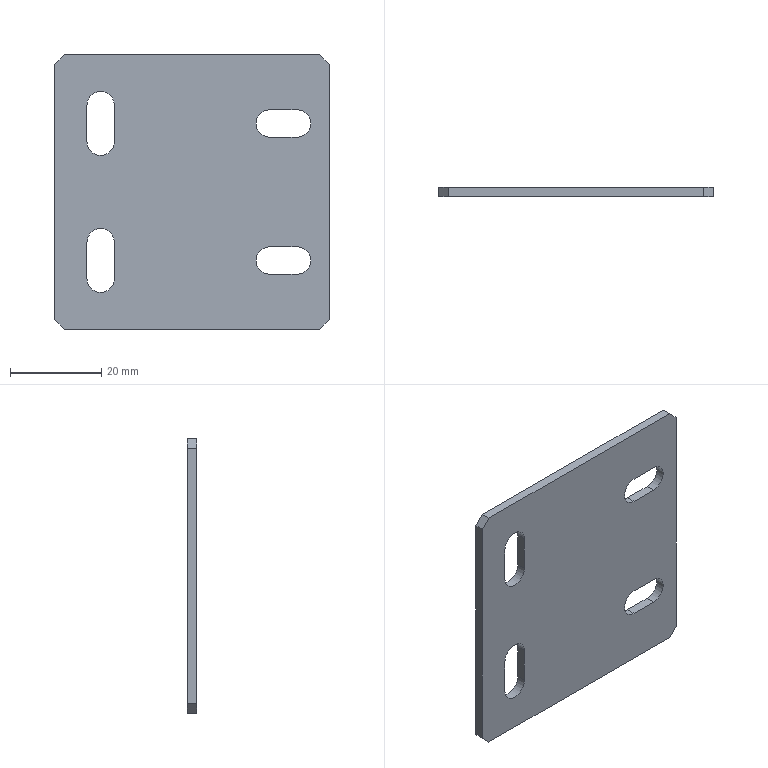Part | NX | features BREP 1 | 1 solid | 28 faces | box 60 x 2 x 60 mm | volume 6622 mm3 | plane 18 | cylinder 10 | commonest cylinder face diameters 6 x10
STEP:
#1=CARTESIAN_POINT('',(30.,-2.,28.));
#2=VERTEX_POINT('',#1);
#3=CARTESIAN_POINT('',(28.,-2.,30.));
#4=VERTEX_POINT('',#3);
#5=CARTESIAN_POINT('',(28.,-2.,30.));
#6=DIRECTION('',(-0.7071,0.,0.7071));
#7=VECTOR('',#6,1000.);
#8=LINE('',#5,#7);
#9=EDGE_CURVE('',#2,#4,#8,.T.);
#10=ORIENTED_EDGE('',*,*,#9,.F.);
#11=CARTESIAN_POINT('',(30.,0.,28.));
#12=VERTEX_POINT('',#11);
#13=CARTESIAN_POINT('',(30.,-2.,28.));
#14=DIRECTION('',(0.,-1.,0.));
#15=VECTOR('',#14,1000.);
#16=LINE('',#13,#15);
#17=EDGE_CURVE('',#12,#2,#16,.T.);
#18=ORIENTED_EDGE('',*,*,#17,.F.);
#19=CARTESIAN_POINT('',(28.,0.,30.));
#20=VERTEX_POINT('',#19);
#21=CARTESIAN_POINT('',(29.,0.,29.));
#22=DIRECTION('',(0.7071,0.,-0.7071));
#23=VECTOR('',#22,1000.);
#24=LINE('',#21,#23);
#25=EDGE_CURVE('',#20,#12,#24,.T.);
#26=ORIENTED_EDGE('',*,*,#25,.F.);
#27=CARTESIAN_POINT('',(28.,-2.,30.));
#28=DIRECTION('',(0.,1.,0.));
#29=VECTOR('',#28,1000.);
#30=LINE('',#27,#29);
#31=EDGE_CURVE('',#4,#20,#30,.T.);
#32=ORIENTED_EDGE('',*,*,#31,.F.);
#33=EDGE_LOOP('',(#10,#18,#26,#32));
#34=FACE_BOUND('',#33,.T.);
#35=CARTESIAN_POINT('',(28.,-2.,30.));
#36=DIRECTION('',(-0.7071,0.,-0.7071));
#37=DIRECTION('',(0.,1.,0.));
#38=AXIS2_PLACEMENT_3D('',#35,#36,#37);
#39=PLANE('',#38);
#40=ADVANCED_FACE('',(#34),#39,.F.);
#41=CARTESIAN_POINT('',(28.,-2.,-30.));
#42=VERTEX_POINT('',#41);
#43=CARTESIAN_POINT('',(30.,-2.,-28.));
#44=VERTEX_POINT('',#43);
#45=CARTESIAN_POINT('',(30.,-2.,-28.));
#46=DIRECTION('',(0.7071,0.,0.7071));
#47=VECTOR('',#46,1000.);
#48=LINE('',#45,#47);
#49=EDGE_CURVE('',#42,#44,#48,.T.);
#50=ORIENTED_EDGE('',*,*,#49,.F.);
#51=CARTESIAN_POINT('',(28.,0.,-30.));
#52=VERTEX_POINT('',#51);
#53=CARTESIAN_POINT('',(28.,-2.,-30.));
#54=DIRECTION('',(0.,-1.,0.));
#55=VECTOR('',#54,1000.);
#56=LINE('',#53,#55);
#57=EDGE_CURVE('',#52,#42,#56,.T.);
#58=ORIENTED_EDGE('',*,*,#57,.F.);
#59=CARTESIAN_POINT('',(30.,0.,-28.));
#60=VERTEX_POINT('',#59);
#61=CARTESIAN_POINT('',(29.,0.,-29.));
#62=DIRECTION('',(-0.7071,0.,-0.7071));
#63=VECTOR('',#62,1000.);
#64=LINE('',#61,#63);
#65=EDGE_CURVE('',#60,#52,#64,.T.);
#66=ORIENTED_EDGE('',*,*,#65,.F.);
#67=CARTESIAN_POINT('',(30.,-2.,-28.));
#68=DIRECTION('',(0.,1.,0.));
#69=VECTOR('',#68,1000.);
#70=LINE('',#67,#69);
#71=EDGE_CURVE('',#44,#60,#70,.T.);
#72=ORIENTED_EDGE('',*,*,#71,.F.);
#73=EDGE_LOOP('',(#50,#58,#66,#72));
#74=FACE_BOUND('',#73,.T.);
#75=CARTESIAN_POINT('',(30.,-2.,-28.));
#76=DIRECTION('',(-0.7071,0.,0.7071));
#77=DIRECTION('',(0.,1.,0.));
#78=AXIS2_PLACEMENT_3D('',#75,#76,#77);
#79=PLANE('',#78);
#80=ADVANCED_FACE('',(#74),#79,.F.);
#81=CARTESIAN_POINT('',(-30.,-2.,-28.));
#82=VERTEX_POINT('',#81);
#83=CARTESIAN_POINT('',(-28.,-2.,-30.));
#84=VERTEX_POINT('',#83);
#85=CARTESIAN_POINT('',(-28.,-2.,-30.));
#86=DIRECTION('',(0.7071,0.,-0.7071));
#87=VECTOR('',#86,1000.);
#88=LINE('',#85,#87);
#89=EDGE_CURVE('',#82,#84,#88,.T.);
#90=ORIENTED_EDGE('',*,*,#89,.F.);
#91=CARTESIAN_POINT('',(-30.,0.,-28.));
#92=VERTEX_POINT('',#91);
#93=CARTESIAN_POINT('',(-30.,-2.,-28.));
#94=DIRECTION('',(0.,-1.,0.));
#95=VECTOR('',#94,1000.);
#96=LINE('',#93,#95);
#97=EDGE_CURVE('',#92,#82,#96,.T.);
#98=ORIENTED_EDGE('',*,*,#97,.F.);
#99=CARTESIAN_POINT('',(-28.,0.,-30.));
#100=VERTEX_POINT('',#99);
#101=CARTESIAN_POINT('',(-29.,0.,-29.));
#102=DIRECTION('',(-0.7071,0.,0.7071));
#103=VECTOR('',#102,1000.);
#104=LINE('',#101,#103);
#105=EDGE_CURVE('',#100,#92,#104,.T.);
#106=ORIENTED_EDGE('',*,*,#105,.F.);
#107=CARTESIAN_POINT('',(-28.,-2.,-30.));
#108=DIRECTION('',(0.,1.,0.));
#109=VECTOR('',#108,1000.);
#110=LINE('',#107,#109);
#111=EDGE_CURVE('',#84,#100,#110,.T.);
#112=ORIENTED_EDGE('',*,*,#111,.F.);
#113=EDGE_LOOP('',(#90,#98,#106,#112));
#114=FACE_BOUND('',#113,.T.);
#115=CARTESIAN_POINT('',(-28.,-2.,-30.));
#116=DIRECTION('',(0.7071,0.,0.7071));
#117=DIRECTION('',(0.,1.,0.));
#118=AXIS2_PLACEMENT_3D('',#115,#116,#117);
#119=PLANE('',#118);
#120=ADVANCED_FACE('',(#114),#119,.F.);
#121=CARTESIAN_POINT('',(-28.,-2.,30.));
#122=VERTEX_POINT('',#121);
#123=CARTESIAN_POINT('',(-30.,-2.,28.));
#124=VERTEX_POINT('',#123);
#125=CARTESIAN_POINT('',(-30.,-2.,28.));
#126=DIRECTION('',(-0.7071,0.,-0.7071));
#127=VECTOR('',#126,1000.);
#128=LINE('',#125,#127);
#129=EDGE_CURVE('',#122,#124,#128,.T.);
#130=ORIENTED_EDGE('',*,*,#129,.F.);
#131=CARTESIAN_POINT('',(-28.,0.,30.));
#132=VERTEX_POINT('',#131);
#133=CARTESIAN_POINT('',(-28.,-2.,30.));
#134=DIRECTION('',(0.,-1.,0.));
#135=VECTOR('',#134,1000.);
#136=LINE('',#133,#135);
#137=EDGE_CURVE('',#132,#122,#136,.T.);
#138=ORIENTED_EDGE('',*,*,#137,.F.);
#139=CARTESIAN_POINT('',(-30.,0.,28.));
#140=VERTEX_POINT('',#139);
#141=CARTESIAN_POINT('',(-29.,0.,29.));
#142=DIRECTION('',(0.7071,0.,0.7071));
#143=VECTOR('',#142,1000.);
#144=LINE('',#141,#143);
#145=EDGE_CURVE('',#140,#132,#144,.T.);
#146=ORIENTED_EDGE('',*,*,#145,.F.);
#147=CARTESIAN_POINT('',(-30.,-2.,28.));
#148=DIRECTION('',(0.,1.,0.));
#149=VECTOR('',#148,1000.);
#150=LINE('',#147,#149);
#151=EDGE_CURVE('',#124,#140,#150,.T.);
#152=ORIENTED_EDGE('',*,*,#151,.F.);
#153=EDGE_LOOP('',(#130,#138,#146,#152));
#154=FACE_BOUND('',#153,.T.);
#155=CARTESIAN_POINT('',(-30.,-2.,28.));
#156=DIRECTION('',(0.7071,0.,-0.7071));
#157=DIRECTION('',(0.,1.,0.));
#158=AXIS2_PLACEMENT_3D('',#155,#156,#157);
#159=PLANE('',#158);
#160=ADVANCED_FACE('',(#154),#159,.F.);
#161=CARTESIAN_POINT('',(-17.,0.,-19.));
#162=VERTEX_POINT('',#161);
#163=CARTESIAN_POINT('',(-17.,-2.,-19.));
#164=VERTEX_POINT('',#163);
#165=CARTESIAN_POINT('',(-17.,-2.,-19.));
#166=DIRECTION('',(0.,-1.,0.));
#167=VECTOR('',#166,1000.);
#168=LINE('',#165,#167);
#169=EDGE_CURVE('',#162,#164,#168,.T.);
#170=ORIENTED_EDGE('',*,*,#169,.T.);
#171=CARTESIAN_POINT('',(-17.,-2.,-11.));
#172=VERTEX_POINT('',#171);
#173=CARTESIAN_POINT('',(-17.,-2.,-11.));
#174=DIRECTION('',(0.,0.,-1.));
#175=VECTOR('',#174,1000.);
#176=LINE('',#173,#175);
#177=EDGE_CURVE('',#172,#164,#176,.T.);
#178=ORIENTED_EDGE('',*,*,#177,.F.);
#179=CARTESIAN_POINT('',(-17.,0.,-11.));
#180=VERTEX_POINT('',#179);
#181=CARTESIAN_POINT('',(-17.,-2.,-11.));
#182=DIRECTION('',(0.,-1.,0.));
#183=VECTOR('',#182,1000.);
#184=LINE('',#181,#183);
#185=EDGE_CURVE('',#180,#172,#184,.T.);
#186=ORIENTED_EDGE('',*,*,#185,.F.);
#187=CARTESIAN_POINT('',(-17.,0.,-11.));
#188=DIRECTION('',(0.,0.,-1.));
#189=VECTOR('',#188,1000.);
#190=LINE('',#187,#189);
#191=EDGE_CURVE('',#180,#162,#190,.T.);
#192=ORIENTED_EDGE('',*,*,#191,.T.);
#193=EDGE_LOOP('',(#170,#178,#186,#192));
#194=FACE_BOUND('',#193,.T.);
#195=CARTESIAN_POINT('',(-17.,-2.,-11.));
#196=DIRECTION('',(1.,0.,0.));
#197=DIRECTION('',(0.,1.,0.));
#198=AXIS2_PLACEMENT_3D('',#195,#196,#197);
#199=PLANE('',#198);
#200=ADVANCED_FACE('',(#194),#199,.F.);
#201=CARTESIAN_POINT('',(-23.,-2.,-19.));
#202=VERTEX_POINT('',#201);
#203=CARTESIAN_POINT('',(-23.,0.,-19.));
#204=VERTEX_POINT('',#203);
#205=CARTESIAN_POINT('',(-23.,0.,-19.));
#206=DIRECTION('',(0.,1.,0.));
#207=VECTOR('',#206,1000.);
#208=LINE('',#205,#207);
#209=EDGE_CURVE('',#202,#204,#208,.T.);
#210=ORIENTED_EDGE('',*,*,#209,.T.);
#211=CARTESIAN_POINT('',(-23.,0.,-11.));
#212=VERTEX_POINT('',#211);
#213=CARTESIAN_POINT('',(-23.,0.,-11.));
#214=DIRECTION('',(0.,0.,-1.));
#215=VECTOR('',#214,1000.);
#216=LINE('',#213,#215);
#217=EDGE_CURVE('',#212,#204,#216,.T.);
#218=ORIENTED_EDGE('',*,*,#217,.F.);
#219=CARTESIAN_POINT('',(-23.,-2.,-11.));
#220=VERTEX_POINT('',#219);
#221=CARTESIAN_POINT('',(-23.,0.,-11.));
#222=DIRECTION('',(0.,-1.,0.));
#223=VECTOR('',#222,1000.);
#224=LINE('',#221,#223);
#225=EDGE_CURVE('',#212,#220,#224,.T.);
#226=ORIENTED_EDGE('',*,*,#225,.T.);
#227=CARTESIAN_POINT('',(-23.,-2.,-11.));
#228=DIRECTION('',(0.,0.,-1.));
#229=VECTOR('',#228,1000.);
#230=LINE('',#227,#229);
#231=EDGE_CURVE('',#220,#202,#230,.T.);
#232=ORIENTED_EDGE('',*,*,#231,.T.);
#233=EDGE_LOOP('',(#210,#218,#226,#232));
#234=FACE_BOUND('',#233,.T.);
#235=CARTESIAN_POINT('',(-23.,0.,-11.));
#236=DIRECTION('',(-1.,0.,0.));
#237=DIRECTION('',(0.,0.,1.));
#238=AXIS2_PLACEMENT_3D('',#235,#236,#237);
#239=PLANE('',#238);
#240=ADVANCED_FACE('',(#234),#239,.F.);
#241=CARTESIAN_POINT('',(-20.,-2.,-8.));
#242=VERTEX_POINT('',#241);
#243=CARTESIAN_POINT('',(-20.,0.,-8.));
#244=VERTEX_POINT('',#243);
#245=CARTESIAN_POINT('',(-20.,0.,-8.));
#246=DIRECTION('',(0.,1.,0.));
#247=VECTOR('',#246,1000.);
#248=LINE('',#245,#247);
#249=EDGE_CURVE('',#242,#244,#248,.T.);
#250=ORIENTED_EDGE('',*,*,#249,.F.);
#251=CARTESIAN_POINT('',(-20.,-2.,-11.));
#252=DIRECTION('',(0.,1.,0.));
#253=DIRECTION('',(0.,0.,1.));
#254=AXIS2_PLACEMENT_3D('',#251,#252,#253);
#255=CIRCLE('',#254,3.);
#256=EDGE_CURVE('',#220,#242,#255,.T.);
#257=ORIENTED_EDGE('',*,*,#256,.F.);
#258=ORIENTED_EDGE('',*,*,#225,.F.);
#259=CARTESIAN_POINT('',(-20.,0.,-11.));
#260=DIRECTION('',(0.,1.,0.));
#261=DIRECTION('',(0.,0.,1.));
#262=AXIS2_PLACEMENT_3D('',#259,#260,#261);
#263=CIRCLE('',#262,3.);
#264=EDGE_CURVE('',#212,#244,#263,.T.);
#265=ORIENTED_EDGE('',*,*,#264,.T.);
#266=EDGE_LOOP('',(#250,#257,#258,#265));
#267=FACE_BOUND('',#266,.T.);
#268=CARTESIAN_POINT('',(-20.,0.,-11.));
#269=DIRECTION('',(0.,1.,0.));
#270=DIRECTION('',(0.,0.,1.));
#271=AXIS2_PLACEMENT_3D('',#268,#269,#270);
#272=CYLINDRICAL_SURFACE('',#271,3.);
#273=ADVANCED_FACE('',(#267),#272,.F.);
#274=CARTESIAN_POINT('',(-20.,-2.,-19.));
#275=DIRECTION('',(0.,1.,0.));
#276=DIRECTION('',(0.,0.,1.));
#277=AXIS2_PLACEMENT_3D('',#274,#275,#276);
#278=CIRCLE('',#277,3.);
#279=EDGE_CURVE('',#164,#202,#278,.T.);
#280=ORIENTED_EDGE('',*,*,#279,.F.);
#281=ORIENTED_EDGE('',*,*,#169,.F.);
#282=CARTESIAN_POINT('',(-20.,0.,-19.));
#283=DIRECTION('',(0.,1.,0.));
#284=DIRECTION('',(0.,0.,1.));
#285=AXIS2_PLACEMENT_3D('',#282,#283,#284);
#286=CIRCLE('',#285,3.);
#287=EDGE_CURVE('',#162,#204,#286,.T.);
#288=ORIENTED_EDGE('',*,*,#287,.T.);
#289=ORIENTED_EDGE('',*,*,#209,.F.);
#290=EDGE_LOOP('',(#280,#281,#288,#289));
#291=FACE_BOUND('',#290,.T.);
#292=CARTESIAN_POINT('',(-20.,0.,-19.));
#293=DIRECTION('',(0.,1.,0.));
#294=DIRECTION('',(0.,0.,1.));
#295=AXIS2_PLACEMENT_3D('',#292,#293,#294);
#296=CYLINDRICAL_SURFACE('',#295,3.);
#297=ADVANCED_FACE('',(#291),#296,.F.);
#298=CARTESIAN_POINT('',(-17.,0.,11.));
#299=VERTEX_POINT('',#298);
#300=CARTESIAN_POINT('',(-17.,-2.,11.));
#301=VERTEX_POINT('',#300);
#302=CARTESIAN_POINT('',(-17.,-2.,11.));
#303=DIRECTION('',(0.,-1.,0.));
#304=VECTOR('',#303,1000.);
#305=LINE('',#302,#304);
#306=EDGE_CURVE('',#299,#301,#305,.T.);
#307=ORIENTED_EDGE('',*,*,#306,.T.);
#308=CARTESIAN_POINT('',(-17.,-2.,19.));
#309=VERTEX_POINT('',#308);
#310=CARTESIAN_POINT('',(-17.,-2.,19.));
#311=DIRECTION('',(0.,0.,-1.));
#312=VECTOR('',#311,1000.);
#313=LINE('',#310,#312);
#314=EDGE_CURVE('',#309,#301,#313,.T.);
#315=ORIENTED_EDGE('',*,*,#314,.F.);
#316=CARTESIAN_POINT('',(-17.,0.,19.));
#317=VERTEX_POINT('',#316);
#318=CARTESIAN_POINT('',(-17.,-2.,19.));
#319=DIRECTION('',(0.,-1.,0.));
#320=VECTOR('',#319,1000.);
#321=LINE('',#318,#320);
#322=EDGE_CURVE('',#317,#309,#321,.T.);
#323=ORIENTED_EDGE('',*,*,#322,.F.);
#324=CARTESIAN_POINT('',(-17.,0.,19.));
#325=DIRECTION('',(0.,0.,-1.));
#326=VECTOR('',#325,1000.);
#327=LINE('',#324,#326);
#328=EDGE_CURVE('',#317,#299,#327,.T.);
#329=ORIENTED_EDGE('',*,*,#328,.T.);
#330=EDGE_LOOP('',(#307,#315,#323,#329));
#331=FACE_BOUND('',#330,.T.);
#332=CARTESIAN_POINT('',(-17.,-2.,19.));
#333=DIRECTION('',(1.,0.,0.));
#334=DIRECTION('',(0.,1.,0.));
#335=AXIS2_PLACEMENT_3D('',#332,#333,#334);
#336=PLANE('',#335);
#337=ADVANCED_FACE('',(#331),#336,.F.);
#338=CARTESIAN_POINT('',(-23.,-2.,11.));
#339=VERTEX_POINT('',#338);
#340=CARTESIAN_POINT('',(-23.,0.,11.));
#341=VERTEX_POINT('',#340);
#342=CARTESIAN_POINT('',(-23.,0.,11.));
#343=DIRECTION('',(0.,1.,0.));
#344=VECTOR('',#343,1000.);
#345=LINE('',#342,#344);
#346=EDGE_CURVE('',#339,#341,#345,.T.);
#347=ORIENTED_EDGE('',*,*,#346,.T.);
#348=CARTESIAN_POINT('',(-23.,0.,19.));
#349=VERTEX_POINT('',#348);
#350=CARTESIAN_POINT('',(-23.,0.,19.));
#351=DIRECTION('',(0.,0.,-1.));
#352=VECTOR('',#351,1000.);
#353=LINE('',#350,#352);
#354=EDGE_CURVE('',#349,#341,#353,.T.);
#355=ORIENTED_EDGE('',*,*,#354,.F.);
#356=CARTESIAN_POINT('',(-23.,-2.,19.));
#357=VERTEX_POINT('',#356);
#358=CARTESIAN_POINT('',(-23.,0.,19.));
#359=DIRECTION('',(0.,-1.,0.));
#360=VECTOR('',#359,1000.);
#361=LINE('',#358,#360);
#362=EDGE_CURVE('',#349,#357,#361,.T.);
#363=ORIENTED_EDGE('',*,*,#362,.T.);
#364=CARTESIAN_POINT('',(-23.,-2.,19.));
#365=DIRECTION('',(0.,0.,-1.));
#366=VECTOR('',#365,1000.);
#367=LINE('',#364,#366);
#368=EDGE_CURVE('',#357,#339,#367,.T.);
#369=ORIENTED_EDGE('',*,*,#368,.T.);
#370=EDGE_LOOP('',(#347,#355,#363,#369));
#371=FACE_BOUND('',#370,.T.);
#372=CARTESIAN_POINT('',(-23.,0.,19.));
#373=DIRECTION('',(-1.,0.,0.));
#374=DIRECTION('',(0.,0.,1.));
#375=AXIS2_PLACEMENT_3D('',#372,#373,#374);
#376=PLANE('',#375);
#377=ADVANCED_FACE('',(#371),#376,.F.);
#378=CARTESIAN_POINT('',(-20.,-2.,22.));
#379=VERTEX_POINT('',#378);
#380=CARTESIAN_POINT('',(-20.,0.,22.));
#381=VERTEX_POINT('',#380);
#382=CARTESIAN_POINT('',(-20.,0.,22.));
#383=DIRECTION('',(0.,1.,0.));
#384=VECTOR('',#383,1000.);
#385=LINE('',#382,#384);
#386=EDGE_CURVE('',#379,#381,#385,.T.);
#387=ORIENTED_EDGE('',*,*,#386,.F.);
#388=CARTESIAN_POINT('',(-20.,-2.,19.));
#389=DIRECTION('',(0.,1.,0.));
#390=DIRECTION('',(0.,0.,1.));
#391=AXIS2_PLACEMENT_3D('',#388,#389,#390);
#392=CIRCLE('',#391,3.);
#393=EDGE_CURVE('',#357,#379,#392,.T.);
#394=ORIENTED_EDGE('',*,*,#393,.F.);
#395=ORIENTED_EDGE('',*,*,#362,.F.);
#396=CARTESIAN_POINT('',(-20.,0.,19.));
#397=DIRECTION('',(0.,1.,0.));
#398=DIRECTION('',(0.,0.,1.));
#399=AXIS2_PLACEMENT_3D('',#396,#397,#398);
#400=CIRCLE('',#399,3.);
#401=EDGE_CURVE('',#349,#381,#400,.T.);
#402=ORIENTED_EDGE('',*,*,#401,.T.);
#403=EDGE_LOOP('',(#387,#394,#395,#402));
#404=FACE_BOUND('',#403,.T.);
#405=CARTESIAN_POINT('',(-20.,0.,19.));
#406=DIRECTION('',(0.,1.,0.));
#407=DIRECTION('',(0.,0.,1.));
#408=AXIS2_PLACEMENT_3D('',#405,#406,#407);
#409=CYLINDRICAL_SURFACE('',#408,3.);
#410=ADVANCED_FACE('',(#404),#409,.F.);
#411=CARTESIAN_POINT('',(-20.,-2.,11.));
#412=DIRECTION('',(0.,1.,0.));
#413=DIRECTION('',(0.,0.,1.));
#414=AXIS2_PLACEMENT_3D('',#411,#412,#413);
#415=CIRCLE('',#414,3.);
#416=EDGE_CURVE('',#301,#339,#415,.T.);
#417=ORIENTED_EDGE('',*,*,#416,.F.);
#418=ORIENTED_EDGE('',*,*,#306,.F.);
#419=CARTESIAN_POINT('',(-20.,0.,11.));
#420=DIRECTION('',(0.,1.,0.));
#421=DIRECTION('',(0.,0.,1.));
#422=AXIS2_PLACEMENT_3D('',#419,#420,#421);
#423=CIRCLE('',#422,3.);
#424=EDGE_CURVE('',#299,#341,#423,.T.);
#425=ORIENTED_EDGE('',*,*,#424,.T.);
#426=ORIENTED_EDGE('',*,*,#346,.F.);
#427=EDGE_LOOP('',(#417,#418,#425,#426));
#428=FACE_BOUND('',#427,.T.);
#429=CARTESIAN_POINT('',(-20.,0.,11.));
#430=DIRECTION('',(0.,1.,0.));
#431=DIRECTION('',(0.,0.,1.));
#432=AXIS2_PLACEMENT_3D('',#429,#430,#431);
#433=CYLINDRICAL_SURFACE('',#432,3.);
#434=ADVANCED_FACE('',(#428),#433,.F.);
#435=CARTESIAN_POINT('',(23.,0.,-12.));
#436=VERTEX_POINT('',#435);
#437=CARTESIAN_POINT('',(23.,-2.,-12.));
#438=VERTEX_POINT('',#437);
#439=CARTESIAN_POINT('',(23.,0.,-12.));
#440=DIRECTION('',(0.,-1.,0.));
#441=VECTOR('',#440,1000.);
#442=LINE('',#439,#441);
#443=EDGE_CURVE('',#436,#438,#442,.T.);
#444=ORIENTED_EDGE('',*,*,#443,.T.);
#445=CARTESIAN_POINT('',(17.,-2.,-12.));
#446=VERTEX_POINT('',#445);
#447=CARTESIAN_POINT('',(17.,-2.,-12.));
#448=DIRECTION('',(1.,0.,0.));
#449=VECTOR('',#448,1000.);
#450=LINE('',#447,#449);
#451=EDGE_CURVE('',#446,#438,#450,.T.);
#452=ORIENTED_EDGE('',*,*,#451,.F.);
#453=CARTESIAN_POINT('',(17.,0.,-12.));
#454=VERTEX_POINT('',#453);
#455=CARTESIAN_POINT('',(17.,0.,-12.));
#456=DIRECTION('',(0.,1.,0.));
#457=VECTOR('',#456,1000.);
#458=LINE('',#455,#457);
#459=EDGE_CURVE('',#446,#454,#458,.T.);
#460=ORIENTED_EDGE('',*,*,#459,.T.);
#461=CARTESIAN_POINT('',(17.,0.,-12.));
#462=DIRECTION('',(1.,0.,0.));
#463=VECTOR('',#462,1000.);
#464=LINE('',#461,#463);
#465=EDGE_CURVE('',#454,#436,#464,.T.);
#466=ORIENTED_EDGE('',*,*,#465,.T.);
#467=EDGE_LOOP('',(#444,#452,#460,#466));
#468=FACE_BOUND('',#467,.T.);
#469=CARTESIAN_POINT('',(17.,0.,-12.));
#470=DIRECTION('',(0.,0.,1.));
#471=DIRECTION('',(1.,0.,0.));
#472=AXIS2_PLACEMENT_3D('',#469,#470,#471);
#473=PLANE('',#472);
#474=ADVANCED_FACE('',(#468),#473,.F.);
#475=CARTESIAN_POINT('',(23.,-2.,-18.));
#476=VERTEX_POINT('',#475);
#477=CARTESIAN_POINT('',(23.,0.,-18.));
#478=VERTEX_POINT('',#477);
#479=CARTESIAN_POINT('',(23.,0.,-18.));
#480=DIRECTION('',(0.,1.,0.));
#481=VECTOR('',#480,1000.);
#482=LINE('',#479,#481);
#483=EDGE_CURVE('',#476,#478,#482,.T.);
#484=ORIENTED_EDGE('',*,*,#483,.T.);
#485=CARTESIAN_POINT('',(17.,0.,-18.));
#486=VERTEX_POINT('',#485);
#487=CARTESIAN_POINT('',(17.,0.,-18.));
#488=DIRECTION('',(1.,0.,0.));
#489=VECTOR('',#488,1000.);
#490=LINE('',#487,#489);
#491=EDGE_CURVE('',#486,#478,#490,.T.);
#492=ORIENTED_EDGE('',*,*,#491,.F.);
#493=CARTESIAN_POINT('',(17.,-2.,-18.));
#494=VERTEX_POINT('',#493);
#495=CARTESIAN_POINT('',(17.,0.,-18.));
#496=DIRECTION('',(0.,-1.,0.));
#497=VECTOR('',#496,1000.);
#498=LINE('',#495,#497);
#499=EDGE_CURVE('',#486,#494,#498,.T.);
#500=ORIENTED_EDGE('',*,*,#499,.T.);
#501=CARTESIAN_POINT('',(17.,-2.,-18.));
#502=DIRECTION('',(1.,0.,0.));
#503=VECTOR('',#502,1000.);
#504=LINE('',#501,#503);
#505=EDGE_CURVE('',#494,#476,#504,.T.);
#506=ORIENTED_EDGE('',*,*,#505,.T.);
#507=EDGE_LOOP('',(#484,#492,#500,#506));
#508=FACE_BOUND('',#507,.T.);
#509=CARTESIAN_POINT('',(17.,0.,-18.));
#510=DIRECTION('',(0.,0.,-1.));
#511=DIRECTION('',(-1.,0.,0.));
#512=AXIS2_PLACEMENT_3D('',#509,#510,#511);
#513=PLANE('',#512);
#514=ADVANCED_FACE('',(#508),#513,.F.);
#515=CARTESIAN_POINT('',(17.,0.,-15.));
#516=DIRECTION('',(0.,1.,0.));
#517=DIRECTION('',(0.,0.,1.));
#518=AXIS2_PLACEMENT_3D('',#515,#516,#517);
#519=CIRCLE('',#518,3.);
#520=EDGE_CURVE('',#486,#454,#519,.T.);
#521=ORIENTED_EDGE('',*,*,#520,.T.);
#522=ORIENTED_EDGE('',*,*,#459,.F.);
#523=CARTESIAN_POINT('',(17.,-2.,-15.));
#524=DIRECTION('',(0.,1.,0.));
#525=DIRECTION('',(0.,0.,1.));
#526=AXIS2_PLACEMENT_3D('',#523,#524,#525);
#527=CIRCLE('',#526,3.);
#528=EDGE_CURVE('',#494,#446,#527,.T.);
#529=ORIENTED_EDGE('',*,*,#528,.F.);
#530=ORIENTED_EDGE('',*,*,#499,.F.);
#531=EDGE_LOOP('',(#521,#522,#529,#530));
#532=FACE_BOUND('',#531,.T.);
#533=CARTESIAN_POINT('',(17.,0.,-15.));
#534=DIRECTION('',(0.,1.,0.));
#535=DIRECTION('',(0.,0.,1.));
#536=AXIS2_PLACEMENT_3D('',#533,#534,#535);
#537=CYLINDRICAL_SURFACE('',#536,3.);
#538=ADVANCED_FACE('',(#532),#537,.F.);
#539=CARTESIAN_POINT('',(23.,-2.,-15.));
#540=DIRECTION('',(0.,1.,0.));
#541=DIRECTION('',(0.,0.,1.));
#542=AXIS2_PLACEMENT_3D('',#539,#540,#541);
#543=CIRCLE('',#542,3.);
#544=EDGE_CURVE('',#438,#476,#543,.T.);
#545=ORIENTED_EDGE('',*,*,#544,.F.);
#546=ORIENTED_EDGE('',*,*,#443,.F.);
#547=CARTESIAN_POINT('',(23.,0.,-15.));
#548=DIRECTION('',(0.,1.,0.));
#549=DIRECTION('',(0.,0.,1.));
#550=AXIS2_PLACEMENT_3D('',#547,#548,#549);
#551=CIRCLE('',#550,3.);
#552=EDGE_CURVE('',#436,#478,#551,.T.);
#553=ORIENTED_EDGE('',*,*,#552,.T.);
#554=ORIENTED_EDGE('',*,*,#483,.F.);
#555=EDGE_LOOP('',(#545,#546,#553,#554));
#556=FACE_BOUND('',#555,.T.);
#557=CARTESIAN_POINT('',(23.,0.,-15.));
#558=DIRECTION('',(0.,1.,0.));
#559=DIRECTION('',(0.,0.,1.));
#560=AXIS2_PLACEMENT_3D('',#557,#558,#559);
#561=CYLINDRICAL_SURFACE('',#560,3.);
#562=ADVANCED_FACE('',(#556),#561,.F.);
#563=CARTESIAN_POINT('',(23.,0.,18.));
#564=VERTEX_POINT('',#563);
#565=CARTESIAN_POINT('',(23.,-2.,18.));
#566=VERTEX_POINT('',#565);
#567=CARTESIAN_POINT('',(23.,0.,18.));
#568=DIRECTION('',(0.,-1.,0.));
#569=VECTOR('',#568,1000.);
#570=LINE('',#567,#569);
#571=EDGE_CURVE('',#564,#566,#570,.T.);
#572=ORIENTED_EDGE('',*,*,#571,.T.);
#573=CARTESIAN_POINT('',(17.,-2.,18.));
#574=VERTEX_POINT('',#573);
#575=CARTESIAN_POINT('',(17.,-2.,18.));
#576=DIRECTION('',(1.,0.,0.));
#577=VECTOR('',#576,1000.);
#578=LINE('',#575,#577);
#579=EDGE_CURVE('',#574,#566,#578,.T.);
#580=ORIENTED_EDGE('',*,*,#579,.F.);
#581=CARTESIAN_POINT('',(17.,0.,18.));
#582=VERTEX_POINT('',#581);
#583=CARTESIAN_POINT('',(17.,0.,18.));
#584=DIRECTION('',(0.,1.,0.));
#585=VECTOR('',#584,1000.);
#586=LINE('',#583,#585);
#587=EDGE_CURVE('',#574,#582,#586,.T.);
#588=ORIENTED_EDGE('',*,*,#587,.T.);
#589=CARTESIAN_POINT('',(17.,0.,18.));
#590=DIRECTION('',(1.,0.,0.));
#591=VECTOR('',#590,1000.);
#592=LINE('',#589,#591);
#593=EDGE_CURVE('',#582,#564,#592,.T.);
#594=ORIENTED_EDGE('',*,*,#593,.T.);
#595=EDGE_LOOP('',(#572,#580,#588,#594));
#596=FACE_BOUND('',#595,.T.);
#597=CARTESIAN_POINT('',(17.,0.,18.));
#598=DIRECTION('',(0.,0.,1.));
#599=DIRECTION('',(1.,0.,0.));
#600=AXIS2_PLACEMENT_3D('',#597,#598,#599);
#601=PLANE('',#600);
#602=ADVANCED_FACE('',(#596),#601,.F.);
#603=CARTESIAN_POINT('',(23.,-2.,12.));
#604=VERTEX_POINT('',#603);
#605=CARTESIAN_POINT('',(23.,0.,12.));
#606=VERTEX_POINT('',#605);
#607=CARTESIAN_POINT('',(23.,0.,12.));
#608=DIRECTION('',(0.,1.,0.));
#609=VECTOR('',#608,1000.);
#610=LINE('',#607,#609);
#611=EDGE_CURVE('',#604,#606,#610,.T.);
#612=ORIENTED_EDGE('',*,*,#611,.T.);
#613=CARTESIAN_POINT('',(17.,0.,12.));
#614=VERTEX_POINT('',#613);
#615=CARTESIAN_POINT('',(17.,0.,12.));
#616=DIRECTION('',(1.,0.,0.));
#617=VECTOR('',#616,1000.);
#618=LINE('',#615,#617);
#619=EDGE_CURVE('',#614,#606,#618,.T.);
#620=ORIENTED_EDGE('',*,*,#619,.F.);
#621=CARTESIAN_POINT('',(17.,-2.,12.));
#622=VERTEX_POINT('',#621);
#623=CARTESIAN_POINT('',(17.,0.,12.));
#624=DIRECTION('',(0.,-1.,0.));
#625=VECTOR('',#624,1000.);
#626=LINE('',#623,#625);
#627=EDGE_CURVE('',#614,#622,#626,.T.);
#628=ORIENTED_EDGE('',*,*,#627,.T.);
#629=CARTESIAN_POINT('',(17.,-2.,12.));
#630=DIRECTION('',(1.,0.,0.));
#631=VECTOR('',#630,1000.);
#632=LINE('',#629,#631);
#633=EDGE_CURVE('',#622,#604,#632,.T.);
#634=ORIENTED_EDGE('',*,*,#633,.T.);
#635=EDGE_LOOP('',(#612,#620,#628,#634));
#636=FACE_BOUND('',#635,.T.);
#637=CARTESIAN_POINT('',(17.,0.,12.));
#638=DIRECTION('',(0.,0.,-1.));
#639=DIRECTION('',(-1.,0.,0.));
#640=AXIS2_PLACEMENT_3D('',#637,#638,#639);
#641=PLANE('',#640);
#642=ADVANCED_FACE('',(#636),#641,.F.);
#643=CARTESIAN_POINT('',(17.,0.,15.));
#644=DIRECTION('',(0.,1.,0.));
#645=DIRECTION('',(0.,0.,1.));
#646=AXIS2_PLACEMENT_3D('',#643,#644,#645);
#647=CIRCLE('',#646,3.);
#648=EDGE_CURVE('',#614,#582,#647,.T.);
#649=ORIENTED_EDGE('',*,*,#648,.T.);
#650=ORIENTED_EDGE('',*,*,#587,.F.);
#651=CARTESIAN_POINT('',(17.,-2.,15.));
#652=DIRECTION('',(0.,1.,0.));
#653=DIRECTION('',(0.,0.,1.));
#654=AXIS2_PLACEMENT_3D('',#651,#652,#653);
#655=CIRCLE('',#654,3.);
#656=EDGE_CURVE('',#622,#574,#655,.T.);
#657=ORIENTED_EDGE('',*,*,#656,.F.);
#658=ORIENTED_EDGE('',*,*,#627,.F.);
#659=EDGE_LOOP('',(#649,#650,#657,#658));
#660=FACE_BOUND('',#659,.T.);
#661=CARTESIAN_POINT('',(17.,0.,15.));
#662=DIRECTION('',(0.,1.,0.));
#663=DIRECTION('',(0.,0.,1.));
#664=AXIS2_PLACEMENT_3D('',#661,#662,#663);
#665=CYLINDRICAL_SURFACE('',#664,3.);
#666=ADVANCED_FACE('',(#660),#665,.F.);
#667=CARTESIAN_POINT('',(23.,-2.,15.));
#668=DIRECTION('',(0.,1.,0.));
#669=DIRECTION('',(0.,0.,1.));
#670=AXIS2_PLACEMENT_3D('',#667,#668,#669);
#671=CIRCLE('',#670,3.);
#672=EDGE_CURVE('',#566,#604,#671,.T.);
#673=ORIENTED_EDGE('',*,*,#672,.F.);
#674=ORIENTED_EDGE('',*,*,#571,.F.);
#675=CARTESIAN_POINT('',(23.,0.,15.));
#676=DIRECTION('',(0.,1.,0.));
#677=DIRECTION('',(0.,0.,1.));
#678=AXIS2_PLACEMENT_3D('',#675,#676,#677);
#679=CIRCLE('',#678,3.);
#680=EDGE_CURVE('',#564,#606,#679,.T.);
#681=ORIENTED_EDGE('',*,*,#680,.T.);
#682=ORIENTED_EDGE('',*,*,#611,.F.);
#683=EDGE_LOOP('',(#673,#674,#681,#682));
#684=FACE_BOUND('',#683,.T.);
#685=CARTESIAN_POINT('',(23.,0.,15.));
#686=DIRECTION('',(0.,1.,0.));
#687=DIRECTION('',(0.,0.,1.));
#688=AXIS2_PLACEMENT_3D('',#685,#686,#687);
#689=CYLINDRICAL_SURFACE('',#688,3.);
#690=ADVANCED_FACE('',(#684),#689,.F.);
#691=CARTESIAN_POINT('',(30.,0.,30.));
#692=DIRECTION('',(1.,0.,0.));
#693=VECTOR('',#692,1000.);
#694=LINE('',#691,#693);
#695=EDGE_CURVE('',#132,#20,#694,.T.);
#696=ORIENTED_EDGE('',*,*,#695,.F.);
#697=ORIENTED_EDGE('',*,*,#137,.T.);
#698=CARTESIAN_POINT('',(30.,-2.,30.));
#699=DIRECTION('',(1.,0.,0.));
#700=VECTOR('',#699,1000.);
#701=LINE('',#698,#700);
#702=EDGE_CURVE('',#122,#4,#701,.T.);
#703=ORIENTED_EDGE('',*,*,#702,.T.);
#704=ORIENTED_EDGE('',*,*,#31,.T.);
#705=EDGE_LOOP('',(#696,#697,#703,#704));
#706=FACE_BOUND('',#705,.T.);
#707=CARTESIAN_POINT('',(30.,-2.,30.));
#708=DIRECTION('',(0.,0.,1.));
#709=DIRECTION('',(1.,0.,0.));
#710=AXIS2_PLACEMENT_3D('',#707,#708,#709);
#711=PLANE('',#710);
#712=ADVANCED_FACE('',(#706),#711,.T.);
#713=CARTESIAN_POINT('',(30.,-2.,30.));
#714=DIRECTION('',(0.,0.,-1.));
#715=VECTOR('',#714,1000.);
#716=LINE('',#713,#715);
#717=EDGE_CURVE('',#2,#44,#716,.T.);
#718=ORIENTED_EDGE('',*,*,#717,.T.);
#719=ORIENTED_EDGE('',*,*,#71,.T.);
#720=CARTESIAN_POINT('',(30.,0.,30.));
#721=DIRECTION('',(0.,0.,-1.));
#722=VECTOR('',#721,1000.);
#723=LINE('',#720,#722);
#724=EDGE_CURVE('',#12,#60,#723,.T.);
#725=ORIENTED_EDGE('',*,*,#724,.F.);
#726=ORIENTED_EDGE('',*,*,#17,.T.);
#727=EDGE_LOOP('',(#718,#719,#725,#726));
#728=FACE_BOUND('',#727,.T.);
#729=CARTESIAN_POINT('',(30.,-2.,30.));
#730=DIRECTION('',(1.,0.,0.));
#731=DIRECTION('',(0.,0.,-1.));
#732=AXIS2_PLACEMENT_3D('',#729,#730,#731);
#733=PLANE('',#732);
#734=ADVANCED_FACE('',(#728),#733,.T.);
#735=CARTESIAN_POINT('',(30.,-2.,-30.));
#736=DIRECTION('',(-1.,0.,0.));
#737=VECTOR('',#736,1000.);
#738=LINE('',#735,#737);
#739=EDGE_CURVE('',#42,#84,#738,.T.);
#740=ORIENTED_EDGE('',*,*,#739,.T.);
#741=ORIENTED_EDGE('',*,*,#111,.T.);
#742=CARTESIAN_POINT('',(30.,0.,-30.));
#743=DIRECTION('',(-1.,0.,0.));
#744=VECTOR('',#743,1000.);
#745=LINE('',#742,#744);
#746=EDGE_CURVE('',#52,#100,#745,.T.);
#747=ORIENTED_EDGE('',*,*,#746,.F.);
#748=ORIENTED_EDGE('',*,*,#57,.T.);
#749=EDGE_LOOP('',(#740,#741,#747,#748));
#750=FACE_BOUND('',#749,.T.);
#751=CARTESIAN_POINT('',(30.,-2.,-30.));
#752=DIRECTION('',(0.,0.,-1.));
#753=DIRECTION('',(-1.,0.,0.));
#754=AXIS2_PLACEMENT_3D('',#751,#752,#753);
#755=PLANE('',#754);
#756=ADVANCED_FACE('',(#750),#755,.T.);
#757=CARTESIAN_POINT('',(-30.,-2.,30.));
#758=DIRECTION('',(0.,0.,1.));
#759=VECTOR('',#758,1000.);
#760=LINE('',#757,#759);
#761=EDGE_CURVE('',#82,#124,#760,.T.);
#762=ORIENTED_EDGE('',*,*,#761,.T.);
#763=ORIENTED_EDGE('',*,*,#151,.T.);
#764=CARTESIAN_POINT('',(-30.,0.,30.));
#765=DIRECTION('',(0.,0.,1.));
#766=VECTOR('',#765,1000.);
#767=LINE('',#764,#766);
#768=EDGE_CURVE('',#92,#140,#767,.T.);
#769=ORIENTED_EDGE('',*,*,#768,.F.);
#770=ORIENTED_EDGE('',*,*,#97,.T.);
#771=EDGE_LOOP('',(#762,#763,#769,#770));
#772=FACE_BOUND('',#771,.T.);
#773=CARTESIAN_POINT('',(-30.,-2.,30.));
#774=DIRECTION('',(-1.,0.,0.));
#775=DIRECTION('',(0.,0.,1.));
#776=AXIS2_PLACEMENT_3D('',#773,#774,#775);
#777=PLANE('',#776);
#778=ADVANCED_FACE('',(#772),#777,.T.);
#779=ORIENTED_EDGE('',*,*,#505,.F.);
#780=ORIENTED_EDGE('',*,*,#528,.T.);
#781=ORIENTED_EDGE('',*,*,#451,.T.);
#782=ORIENTED_EDGE('',*,*,#544,.T.);
#783=EDGE_LOOP('',(#779,#780,#781,#782));
#784=FACE_BOUND('',#783,.T.);
#785=ORIENTED_EDGE('',*,*,#702,.F.);
#786=ORIENTED_EDGE('',*,*,#129,.T.);
#787=ORIENTED_EDGE('',*,*,#761,.F.);
#788=ORIENTED_EDGE('',*,*,#89,.T.);
#789=ORIENTED_EDGE('',*,*,#739,.F.);
#790=ORIENTED_EDGE('',*,*,#49,.T.);
#791=ORIENTED_EDGE('',*,*,#717,.F.);
#792=ORIENTED_EDGE('',*,*,#9,.T.);
#793=EDGE_LOOP('',(#785,#786,#787,#788,#789,#790,#791,#792));
#794=FACE_BOUND('',#793,.T.);
#795=ORIENTED_EDGE('',*,*,#633,.F.);
#796=ORIENTED_EDGE('',*,*,#656,.T.);
#797=ORIENTED_EDGE('',*,*,#579,.T.);
#798=ORIENTED_EDGE('',*,*,#672,.T.);
#799=EDGE_LOOP('',(#795,#796,#797,#798));
#800=FACE_BOUND('',#799,.T.);
#801=ORIENTED_EDGE('',*,*,#393,.T.);
#802=CARTESIAN_POINT('',(-20.,-2.,19.));
#803=DIRECTION('',(0.,1.,0.));
#804=DIRECTION('',(0.,0.,1.));
#805=AXIS2_PLACEMENT_3D('',#802,#803,#804);
#806=CIRCLE('',#805,3.);
#807=EDGE_CURVE('',#379,#309,#806,.T.);
#808=ORIENTED_EDGE('',*,*,#807,.T.);
#809=ORIENTED_EDGE('',*,*,#314,.T.);
#810=ORIENTED_EDGE('',*,*,#416,.T.);
#811=ORIENTED_EDGE('',*,*,#368,.F.);
#812=EDGE_LOOP('',(#801,#808,#809,#810,#811));
#813=FACE_BOUND('',#812,.T.);
#814=ORIENTED_EDGE('',*,*,#177,.T.);
#815=ORIENTED_EDGE('',*,*,#279,.T.);
#816=ORIENTED_EDGE('',*,*,#231,.F.);
#817=ORIENTED_EDGE('',*,*,#256,.T.);
#818=CARTESIAN_POINT('',(-20.,-2.,-11.));
#819=DIRECTION('',(0.,1.,0.));
#820=DIRECTION('',(0.,0.,1.));
#821=AXIS2_PLACEMENT_3D('',#818,#819,#820);
#822=CIRCLE('',#821,3.);
#823=EDGE_CURVE('',#242,#172,#822,.T.);
#824=ORIENTED_EDGE('',*,*,#823,.T.);
#825=EDGE_LOOP('',(#814,#815,#816,#817,#824));
#826=FACE_BOUND('',#825,.T.);
#827=CARTESIAN_POINT('',(0.,-2.,0.));
#828=DIRECTION('',(0.,1.,0.));
#829=DIRECTION('',(0.,0.,1.));
#830=AXIS2_PLACEMENT_3D('',#827,#828,#829);
#831=PLANE('',#830);
#832=ADVANCED_FACE('',(#784,#794,#800,#813,#826),#831,.F.);
#833=ORIENTED_EDGE('',*,*,#401,.F.);
#834=ORIENTED_EDGE('',*,*,#354,.T.);
#835=ORIENTED_EDGE('',*,*,#424,.F.);
#836=ORIENTED_EDGE('',*,*,#328,.F.);
#837=CARTESIAN_POINT('',(-20.,0.,19.));
#838=DIRECTION('',(0.,1.,0.));
#839=DIRECTION('',(0.,0.,1.));
#840=AXIS2_PLACEMENT_3D('',#837,#838,#839);
#841=CIRCLE('',#840,3.);
#842=EDGE_CURVE('',#381,#317,#841,.T.);
#843=ORIENTED_EDGE('',*,*,#842,.F.);
#844=EDGE_LOOP('',(#833,#834,#835,#836,#843));
#845=FACE_BOUND('',#844,.T.);
#846=ORIENTED_EDGE('',*,*,#768,.T.);
#847=ORIENTED_EDGE('',*,*,#145,.T.);
#848=ORIENTED_EDGE('',*,*,#695,.T.);
#849=ORIENTED_EDGE('',*,*,#25,.T.);
#850=ORIENTED_EDGE('',*,*,#724,.T.);
#851=ORIENTED_EDGE('',*,*,#65,.T.);
#852=ORIENTED_EDGE('',*,*,#746,.T.);
#853=ORIENTED_EDGE('',*,*,#105,.T.);
#854=EDGE_LOOP('',(#846,#847,#848,#849,#850,#851,#852,#853));
#855=FACE_BOUND('',#854,.T.);
#856=ORIENTED_EDGE('',*,*,#648,.F.);
#857=ORIENTED_EDGE('',*,*,#619,.T.);
#858=ORIENTED_EDGE('',*,*,#680,.F.);
#859=ORIENTED_EDGE('',*,*,#593,.F.);
#860=EDGE_LOOP('',(#856,#857,#858,#859));
#861=FACE_BOUND('',#860,.T.);
#862=ORIENTED_EDGE('',*,*,#491,.T.);
#863=ORIENTED_EDGE('',*,*,#552,.F.);
#864=ORIENTED_EDGE('',*,*,#465,.F.);
#865=ORIENTED_EDGE('',*,*,#520,.F.);
#866=EDGE_LOOP('',(#862,#863,#864,#865));
#867=FACE_BOUND('',#866,.T.);
#868=ORIENTED_EDGE('',*,*,#287,.F.);
#869=ORIENTED_EDGE('',*,*,#191,.F.);
#870=CARTESIAN_POINT('',(-20.,0.,-11.));
#871=DIRECTION('',(0.,1.,0.));
#872=DIRECTION('',(0.,0.,1.));
#873=AXIS2_PLACEMENT_3D('',#870,#871,#872);
#874=CIRCLE('',#873,3.);
#875=EDGE_CURVE('',#244,#180,#874,.T.);
#876=ORIENTED_EDGE('',*,*,#875,.F.);
#877=ORIENTED_EDGE('',*,*,#264,.F.);
#878=ORIENTED_EDGE('',*,*,#217,.T.);
#879=EDGE_LOOP('',(#868,#869,#876,#877,#878));
#880=FACE_BOUND('',#879,.T.);
#881=CARTESIAN_POINT('',(0.,0.,0.));
#882=DIRECTION('',(0.,1.,0.));
#883=DIRECTION('',(0.,0.,1.));
#884=AXIS2_PLACEMENT_3D('',#881,#882,#883);
#885=PLANE('',#884);
#886=ADVANCED_FACE('',(#845,#855,#861,#867,#880),#885,.T.);
#887=ORIENTED_EDGE('',*,*,#807,.F.);
#888=ORIENTED_EDGE('',*,*,#386,.T.);
#889=ORIENTED_EDGE('',*,*,#842,.T.);
#890=ORIENTED_EDGE('',*,*,#322,.T.);
#891=EDGE_LOOP('',(#887,#888,#889,#890));
#892=FACE_BOUND('',#891,.T.);
#893=CARTESIAN_POINT('',(-20.,0.,19.));
#894=DIRECTION('',(0.,1.,0.));
#895=DIRECTION('',(0.,0.,1.));
#896=AXIS2_PLACEMENT_3D('',#893,#894,#895);
#897=CYLINDRICAL_SURFACE('',#896,3.);
#898=ADVANCED_FACE('',(#892),#897,.F.);
#899=ORIENTED_EDGE('',*,*,#823,.F.);
#900=ORIENTED_EDGE('',*,*,#249,.T.);
#901=ORIENTED_EDGE('',*,*,#875,.T.);
#902=ORIENTED_EDGE('',*,*,#185,.T.);
#903=EDGE_LOOP('',(#899,#900,#901,#902));
#904=FACE_BOUND('',#903,.T.);
#905=CARTESIAN_POINT('',(-20.,0.,-11.));
#906=DIRECTION('',(0.,1.,0.));
#907=DIRECTION('',(0.,0.,1.));
#908=AXIS2_PLACEMENT_3D('',#905,#906,#907);
#909=CYLINDRICAL_SURFACE('',#908,3.);
#910=ADVANCED_FACE('',(#904),#909,.F.);
#911=CLOSED_SHELL('',(#40,#80,#120,#160,#200,#240,#273,#297,#337,#377,#410,#434,#474,#514,#538,#562,#602,#642,#666,#690,#712,#734,#756,#778,#832,#886,#898,#910));
#912=MANIFOLD_SOLID_BREP('',#911);
#913=(LENGTH_UNIT()NAMED_UNIT(*)SI_UNIT(.MILLI.,.METRE.));
#914=UNCERTAINTY_MEASURE_WITH_UNIT(LENGTH_MEASURE(0.00001),#913,'','');
#915=(NAMED_UNIT(*)PLANE_ANGLE_UNIT()SI_UNIT($,.RADIAN.));
#916=(NAMED_UNIT(*)SI_UNIT($,.STERADIAN.)SOLID_ANGLE_UNIT());
#917=(GEOMETRIC_REPRESENTATION_CONTEXT(3)GLOBAL_UNCERTAINTY_ASSIGNED_CONTEXT((#914))GLOBAL_UNIT_ASSIGNED_CONTEXT((#913,#915,#916))REPRESENTATION_CONTEXT('',''));
#918=ADVANCED_BREP_SHAPE_REPRESENTATION('',(#912),#917);